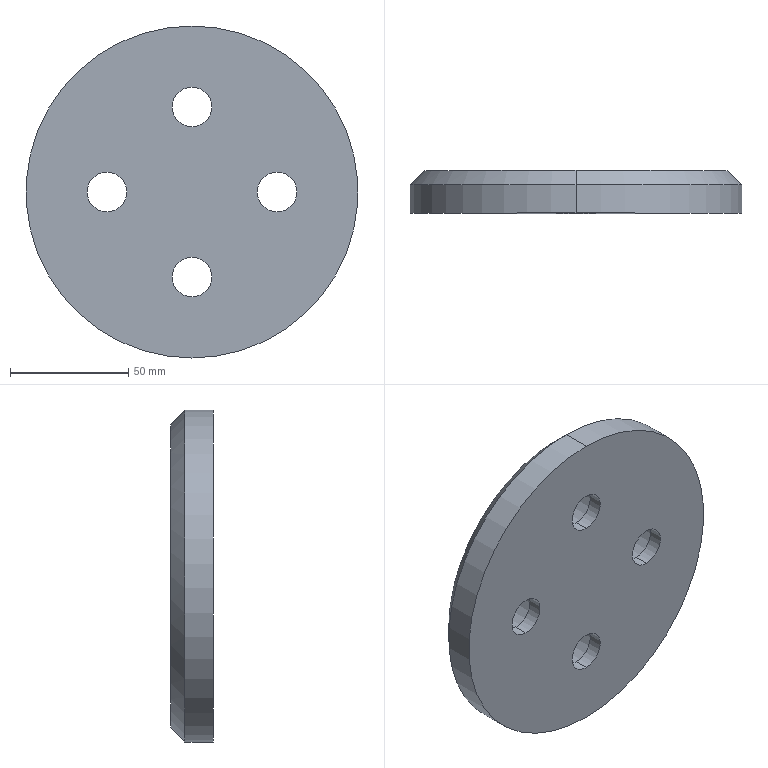Part | SolidWorks | features BaseBody 1, Scale 1 | 1 solid | 26 faces | box 140.4 x 18 x 140.4 mm | volume 234372 mm3 | cylinder 18 | plane 6 | cone 2 | commonest cylinder face diameters 16.8 x8 28.8 x8 140.4 x2
STEP:
#1=CARTESIAN_POINT('',(-36.,4.582,8.4));
#2=VERTEX_POINT('',#1);
#3=CARTESIAN_POINT('',(-36.,4.582,-8.4));
#4=VERTEX_POINT('',#3);
#5=CARTESIAN_POINT('',(-36.,4.582,0.));
#6=DIRECTION('',(0.,-1.,0.));
#7=DIRECTION('',(0.,0.,-1.));
#8=AXIS2_PLACEMENT_3D('',#5,#6,#7);
#9=CIRCLE('',#8,8.4);
#10=EDGE_CURVE('',#2,#4,#9,.T.);
#11=ORIENTED_EDGE('',*,*,#10,.F.);
#12=CARTESIAN_POINT('',(-36.,-1.418,8.4));
#13=VERTEX_POINT('',#12);
#14=CARTESIAN_POINT('',(-36.,16.582,8.4));
#15=DIRECTION('',(0.,-1.,0.));
#16=VECTOR('',#15,1000.);
#17=LINE('',#14,#16);
#18=EDGE_CURVE('',#2,#13,#17,.T.);
#19=ORIENTED_EDGE('',*,*,#18,.T.);
#20=CARTESIAN_POINT('',(-36.,-1.418,-8.4));
#21=VERTEX_POINT('',#20);
#22=CARTESIAN_POINT('',(-36.,-1.418,0.));
#23=DIRECTION('',(0.,-1.,0.));
#24=DIRECTION('',(0.,0.,-1.));
#25=AXIS2_PLACEMENT_3D('',#22,#23,#24);
#26=CIRCLE('',#25,8.4);
#27=EDGE_CURVE('',#13,#21,#26,.T.);
#28=ORIENTED_EDGE('',*,*,#27,.T.);
#29=CARTESIAN_POINT('',(-36.,16.582,-8.4));
#30=DIRECTION('',(0.,-1.,0.));
#31=VECTOR('',#30,1000.);
#32=LINE('',#29,#31);
#33=EDGE_CURVE('',#4,#21,#32,.T.);
#34=ORIENTED_EDGE('',*,*,#33,.F.);
#35=EDGE_LOOP('',(#11,#19,#28,#34));
#36=FACE_OUTER_BOUND('',#35,.T.);
#37=CARTESIAN_POINT('',(-36.,16.582,0.));
#38=DIRECTION('',(0.,-1.,0.));
#39=DIRECTION('',(0.,0.,-1.));
#40=AXIS2_PLACEMENT_3D('',#37,#38,#39);
#41=CYLINDRICAL_SURFACE('',#40,8.4);
#42=ADVANCED_FACE('',(#36),#41,.F.);
#43=CARTESIAN_POINT('',(0.,4.582,44.4));
#44=VERTEX_POINT('',#43);
#45=CARTESIAN_POINT('',(0.,4.582,27.6));
#46=VERTEX_POINT('',#45);
#47=CARTESIAN_POINT('',(0.,4.582,36.));
#48=DIRECTION('',(0.,-1.,0.));
#49=DIRECTION('',(0.,0.,-1.));
#50=AXIS2_PLACEMENT_3D('',#47,#48,#49);
#51=CIRCLE('',#50,8.4);
#52=EDGE_CURVE('',#44,#46,#51,.T.);
#53=ORIENTED_EDGE('',*,*,#52,.F.);
#54=CARTESIAN_POINT('',(0.,-1.418,44.4));
#55=VERTEX_POINT('',#54);
#56=CARTESIAN_POINT('',(0.,16.582,44.4));
#57=DIRECTION('',(0.,-1.,0.));
#58=VECTOR('',#57,1000.);
#59=LINE('',#56,#58);
#60=EDGE_CURVE('',#44,#55,#59,.T.);
#61=ORIENTED_EDGE('',*,*,#60,.T.);
#62=CARTESIAN_POINT('',(0.,-1.418,27.6));
#63=VERTEX_POINT('',#62);
#64=CARTESIAN_POINT('',(0.,-1.418,36.));
#65=DIRECTION('',(0.,-1.,0.));
#66=DIRECTION('',(0.,0.,-1.));
#67=AXIS2_PLACEMENT_3D('',#64,#65,#66);
#68=CIRCLE('',#67,8.4);
#69=EDGE_CURVE('',#55,#63,#68,.T.);
#70=ORIENTED_EDGE('',*,*,#69,.T.);
#71=CARTESIAN_POINT('',(0.,16.582,27.6));
#72=DIRECTION('',(0.,-1.,0.));
#73=VECTOR('',#72,1000.);
#74=LINE('',#71,#73);
#75=EDGE_CURVE('',#46,#63,#74,.T.);
#76=ORIENTED_EDGE('',*,*,#75,.F.);
#77=EDGE_LOOP('',(#53,#61,#70,#76));
#78=FACE_OUTER_BOUND('',#77,.T.);
#79=CARTESIAN_POINT('',(0.,16.582,36.));
#80=DIRECTION('',(0.,-1.,0.));
#81=DIRECTION('',(0.,0.,-1.));
#82=AXIS2_PLACEMENT_3D('',#79,#80,#81);
#83=CYLINDRICAL_SURFACE('',#82,8.4);
#84=ADVANCED_FACE('',(#78),#83,.F.);
#85=CARTESIAN_POINT('',(36.,4.582,8.4));
#86=VERTEX_POINT('',#85);
#87=CARTESIAN_POINT('',(36.,4.582,-8.4));
#88=VERTEX_POINT('',#87);
#89=CARTESIAN_POINT('',(36.,4.582,0.));
#90=DIRECTION('',(0.,-1.,0.));
#91=DIRECTION('',(0.,0.,-1.));
#92=AXIS2_PLACEMENT_3D('',#89,#90,#91);
#93=CIRCLE('',#92,8.4);
#94=EDGE_CURVE('',#86,#88,#93,.T.);
#95=ORIENTED_EDGE('',*,*,#94,.F.);
#96=CARTESIAN_POINT('',(36.,-1.418,8.4));
#97=VERTEX_POINT('',#96);
#98=CARTESIAN_POINT('',(36.,16.582,8.4));
#99=DIRECTION('',(0.,-1.,0.));
#100=VECTOR('',#99,1000.);
#101=LINE('',#98,#100);
#102=EDGE_CURVE('',#86,#97,#101,.T.);
#103=ORIENTED_EDGE('',*,*,#102,.T.);
#104=CARTESIAN_POINT('',(36.,-1.418,-8.4));
#105=VERTEX_POINT('',#104);
#106=CARTESIAN_POINT('',(36.,-1.418,0.));
#107=DIRECTION('',(0.,-1.,0.));
#108=DIRECTION('',(0.,0.,-1.));
#109=AXIS2_PLACEMENT_3D('',#106,#107,#108);
#110=CIRCLE('',#109,8.4);
#111=EDGE_CURVE('',#97,#105,#110,.T.);
#112=ORIENTED_EDGE('',*,*,#111,.T.);
#113=CARTESIAN_POINT('',(36.,16.582,-8.4));
#114=DIRECTION('',(0.,-1.,0.));
#115=VECTOR('',#114,1000.);
#116=LINE('',#113,#115);
#117=EDGE_CURVE('',#88,#105,#116,.T.);
#118=ORIENTED_EDGE('',*,*,#117,.F.);
#119=EDGE_LOOP('',(#95,#103,#112,#118));
#120=FACE_OUTER_BOUND('',#119,.T.);
#121=CARTESIAN_POINT('',(36.,16.582,0.));
#122=DIRECTION('',(0.,-1.,0.));
#123=DIRECTION('',(0.,0.,-1.));
#124=AXIS2_PLACEMENT_3D('',#121,#122,#123);
#125=CYLINDRICAL_SURFACE('',#124,8.4);
#126=ADVANCED_FACE('',(#120),#125,.F.);
#127=CARTESIAN_POINT('',(0.,4.582,-27.6));
#128=VERTEX_POINT('',#127);
#129=CARTESIAN_POINT('',(0.,4.582,-44.4));
#130=VERTEX_POINT('',#129);
#131=CARTESIAN_POINT('',(0.,4.582,-36.));
#132=DIRECTION('',(0.,-1.,0.));
#133=DIRECTION('',(0.,0.,-1.));
#134=AXIS2_PLACEMENT_3D('',#131,#132,#133);
#135=CIRCLE('',#134,8.4);
#136=EDGE_CURVE('',#128,#130,#135,.T.);
#137=ORIENTED_EDGE('',*,*,#136,.F.);
#138=CARTESIAN_POINT('',(0.,-1.418,-27.6));
#139=VERTEX_POINT('',#138);
#140=CARTESIAN_POINT('',(0.,16.582,-27.6));
#141=DIRECTION('',(0.,-1.,0.));
#142=VECTOR('',#141,1000.);
#143=LINE('',#140,#142);
#144=EDGE_CURVE('',#128,#139,#143,.T.);
#145=ORIENTED_EDGE('',*,*,#144,.T.);
#146=CARTESIAN_POINT('',(0.,-1.418,-44.4));
#147=VERTEX_POINT('',#146);
#148=CARTESIAN_POINT('',(0.,-1.418,-36.));
#149=DIRECTION('',(0.,-1.,0.));
#150=DIRECTION('',(0.,0.,-1.));
#151=AXIS2_PLACEMENT_3D('',#148,#149,#150);
#152=CIRCLE('',#151,8.4);
#153=EDGE_CURVE('',#139,#147,#152,.T.);
#154=ORIENTED_EDGE('',*,*,#153,.T.);
#155=CARTESIAN_POINT('',(0.,16.582,-44.4));
#156=DIRECTION('',(0.,-1.,0.));
#157=VECTOR('',#156,1000.);
#158=LINE('',#155,#157);
#159=EDGE_CURVE('',#130,#147,#158,.T.);
#160=ORIENTED_EDGE('',*,*,#159,.F.);
#161=EDGE_LOOP('',(#137,#145,#154,#160));
#162=FACE_OUTER_BOUND('',#161,.T.);
#163=CARTESIAN_POINT('',(0.,16.582,-36.));
#164=DIRECTION('',(0.,-1.,0.));
#165=DIRECTION('',(0.,0.,-1.));
#166=AXIS2_PLACEMENT_3D('',#163,#164,#165);
#167=CYLINDRICAL_SURFACE('',#166,8.4);
#168=ADVANCED_FACE('',(#162),#167,.F.);
#169=CARTESIAN_POINT('',(0.,10.582,-70.2));
#170=VERTEX_POINT('',#169);
#171=CARTESIAN_POINT('',(0.,10.582,70.2));
#172=VERTEX_POINT('',#171);
#173=CARTESIAN_POINT('',(0.,10.582,0.));
#174=DIRECTION('',(0.,-1.,0.));
#175=DIRECTION('',(0.,0.,-1.));
#176=AXIS2_PLACEMENT_3D('',#173,#174,#175);
#177=CIRCLE('',#176,70.2);
#178=EDGE_CURVE('',#170,#172,#177,.T.);
#179=ORIENTED_EDGE('',*,*,#178,.T.);
#180=CARTESIAN_POINT('',(0.,-1.418,70.2));
#181=VERTEX_POINT('',#180);
#182=CARTESIAN_POINT('',(0.,16.582,70.2));
#183=DIRECTION('',(0.,-1.,0.));
#184=VECTOR('',#183,1000.);
#185=LINE('',#182,#184);
#186=EDGE_CURVE('',#172,#181,#185,.T.);
#187=ORIENTED_EDGE('',*,*,#186,.T.);
#188=CARTESIAN_POINT('',(0.,-1.418,-70.2));
#189=VERTEX_POINT('',#188);
#190=CARTESIAN_POINT('',(0.,-1.418,0.));
#191=DIRECTION('',(0.,1.,0.));
#192=DIRECTION('',(0.,0.,-1.));
#193=AXIS2_PLACEMENT_3D('',#190,#191,#192);
#194=CIRCLE('',#193,70.2);
#195=EDGE_CURVE('',#181,#189,#194,.T.);
#196=ORIENTED_EDGE('',*,*,#195,.T.);
#197=CARTESIAN_POINT('',(0.,16.582,-70.2));
#198=DIRECTION('',(0.,-1.,0.));
#199=VECTOR('',#198,1000.);
#200=LINE('',#197,#199);
#201=EDGE_CURVE('',#170,#189,#200,.T.);
#202=ORIENTED_EDGE('',*,*,#201,.F.);
#203=EDGE_LOOP('',(#179,#187,#196,#202));
#204=FACE_OUTER_BOUND('',#203,.T.);
#205=CARTESIAN_POINT('',(0.,16.582,0.));
#206=DIRECTION('',(0.,-1.,0.));
#207=DIRECTION('',(0.,0.,-1.));
#208=AXIS2_PLACEMENT_3D('',#205,#206,#207);
#209=CYLINDRICAL_SURFACE('',#208,70.2);
#210=ADVANCED_FACE('',(#204),#209,.T.);
#211=CARTESIAN_POINT('',(0.,16.582,-64.2));
#212=VERTEX_POINT('',#211);
#213=CARTESIAN_POINT('',(0.,16.582,64.2));
#214=VERTEX_POINT('',#213);
#215=CARTESIAN_POINT('',(0.,16.582,0.));
#216=DIRECTION('',(0.,-1.,0.));
#217=DIRECTION('',(0.,0.,-1.));
#218=AXIS2_PLACEMENT_3D('',#215,#216,#217);
#219=CIRCLE('',#218,64.2);
#220=EDGE_CURVE('',#212,#214,#219,.T.);
#221=ORIENTED_EDGE('',*,*,#220,.T.);
#222=CARTESIAN_POINT('',(0.,10.582,70.2));
#223=DIRECTION('',(0.,-0.7071,0.7071));
#224=VECTOR('',#223,1000.);
#225=LINE('',#222,#224);
#226=EDGE_CURVE('',#214,#172,#225,.T.);
#227=ORIENTED_EDGE('',*,*,#226,.T.);
#228=ORIENTED_EDGE('',*,*,#178,.F.);
#229=CARTESIAN_POINT('',(0.,10.582,-70.2));
#230=DIRECTION('',(0.,-0.7071,-0.7071));
#231=VECTOR('',#230,1000.);
#232=LINE('',#229,#231);
#233=EDGE_CURVE('',#212,#170,#232,.T.);
#234=ORIENTED_EDGE('',*,*,#233,.F.);
#235=EDGE_LOOP('',(#221,#227,#228,#234));
#236=FACE_OUTER_BOUND('',#235,.T.);
#237=CARTESIAN_POINT('',(0.,10.582,0.));
#238=DIRECTION('',(0.,-1.,0.));
#239=DIRECTION('',(0.,0.,-1.));
#240=AXIS2_PLACEMENT_3D('',#237,#238,#239);
#241=CONICAL_SURFACE('',#240,70.2,0.7854);
#242=ADVANCED_FACE('',(#236),#241,.T.);
#243=CARTESIAN_POINT('',(-36.,4.582,-14.4));
#244=VERTEX_POINT('',#243);
#245=CARTESIAN_POINT('',(-36.,4.582,14.4));
#246=VERTEX_POINT('',#245);
#247=CARTESIAN_POINT('',(-36.,4.582,0.));
#248=DIRECTION('',(0.,1.,0.));
#249=DIRECTION('',(0.,0.,1.));
#250=AXIS2_PLACEMENT_3D('',#247,#248,#249);
#251=CIRCLE('',#250,14.4);
#252=EDGE_CURVE('',#244,#246,#251,.T.);
#253=ORIENTED_EDGE('',*,*,#252,.F.);
#254=CARTESIAN_POINT('',(-36.,16.582,-14.4));
#255=VERTEX_POINT('',#254);
#256=CARTESIAN_POINT('',(-36.,4.582,-14.4));
#257=DIRECTION('',(0.,1.,0.));
#258=VECTOR('',#257,1000.);
#259=LINE('',#256,#258);
#260=EDGE_CURVE('',#244,#255,#259,.T.);
#261=ORIENTED_EDGE('',*,*,#260,.T.);
#262=CARTESIAN_POINT('',(-36.,16.582,14.4));
#263=VERTEX_POINT('',#262);
#264=CARTESIAN_POINT('',(-36.,16.582,0.));
#265=DIRECTION('',(0.,-1.,0.));
#266=DIRECTION('',(0.,0.,1.));
#267=AXIS2_PLACEMENT_3D('',#264,#265,#266);
#268=CIRCLE('',#267,14.4);
#269=EDGE_CURVE('',#263,#255,#268,.T.);
#270=ORIENTED_EDGE('',*,*,#269,.F.);
#271=CARTESIAN_POINT('',(-36.,4.582,14.4));
#272=DIRECTION('',(0.,1.,0.));
#273=VECTOR('',#272,1000.);
#274=LINE('',#271,#273);
#275=EDGE_CURVE('',#246,#263,#274,.T.);
#276=ORIENTED_EDGE('',*,*,#275,.F.);
#277=EDGE_LOOP('',(#253,#261,#270,#276));
#278=FACE_OUTER_BOUND('',#277,.T.);
#279=CARTESIAN_POINT('',(-36.,4.582,0.));
#280=DIRECTION('',(0.,1.,0.));
#281=DIRECTION('',(0.,0.,1.));
#282=AXIS2_PLACEMENT_3D('',#279,#280,#281);
#283=CYLINDRICAL_SURFACE('',#282,14.4);
#284=ADVANCED_FACE('',(#278),#283,.F.);
#285=CARTESIAN_POINT('',(0.,4.582,21.6));
#286=VERTEX_POINT('',#285);
#287=CARTESIAN_POINT('',(0.,4.582,50.4));
#288=VERTEX_POINT('',#287);
#289=CARTESIAN_POINT('',(0.,4.582,36.));
#290=DIRECTION('',(0.,1.,0.));
#291=DIRECTION('',(0.,0.,1.));
#292=AXIS2_PLACEMENT_3D('',#289,#290,#291);
#293=CIRCLE('',#292,14.4);
#294=EDGE_CURVE('',#286,#288,#293,.T.);
#295=ORIENTED_EDGE('',*,*,#294,.F.);
#296=CARTESIAN_POINT('',(0.,16.582,21.6));
#297=VERTEX_POINT('',#296);
#298=CARTESIAN_POINT('',(0.,4.582,21.6));
#299=DIRECTION('',(0.,1.,0.));
#300=VECTOR('',#299,1000.);
#301=LINE('',#298,#300);
#302=EDGE_CURVE('',#286,#297,#301,.T.);
#303=ORIENTED_EDGE('',*,*,#302,.T.);
#304=CARTESIAN_POINT('',(0.,16.582,50.4));
#305=VERTEX_POINT('',#304);
#306=CARTESIAN_POINT('',(0.,16.582,36.));
#307=DIRECTION('',(0.,-1.,0.));
#308=DIRECTION('',(0.,0.,1.));
#309=AXIS2_PLACEMENT_3D('',#306,#307,#308);
#310=CIRCLE('',#309,14.4);
#311=EDGE_CURVE('',#305,#297,#310,.T.);
#312=ORIENTED_EDGE('',*,*,#311,.F.);
#313=CARTESIAN_POINT('',(0.,4.582,50.4));
#314=DIRECTION('',(0.,1.,0.));
#315=VECTOR('',#314,1000.);
#316=LINE('',#313,#315);
#317=EDGE_CURVE('',#288,#305,#316,.T.);
#318=ORIENTED_EDGE('',*,*,#317,.F.);
#319=EDGE_LOOP('',(#295,#303,#312,#318));
#320=FACE_OUTER_BOUND('',#319,.T.);
#321=CARTESIAN_POINT('',(0.,4.582,36.));
#322=DIRECTION('',(0.,1.,0.));
#323=DIRECTION('',(0.,0.,1.));
#324=AXIS2_PLACEMENT_3D('',#321,#322,#323);
#325=CYLINDRICAL_SURFACE('',#324,14.4);
#326=ADVANCED_FACE('',(#320),#325,.F.);
#327=CARTESIAN_POINT('',(36.,4.582,-14.4));
#328=VERTEX_POINT('',#327);
#329=CARTESIAN_POINT('',(36.,4.582,14.4));
#330=VERTEX_POINT('',#329);
#331=CARTESIAN_POINT('',(36.,4.582,0.));
#332=DIRECTION('',(0.,1.,0.));
#333=DIRECTION('',(0.,0.,1.));
#334=AXIS2_PLACEMENT_3D('',#331,#332,#333);
#335=CIRCLE('',#334,14.4);
#336=EDGE_CURVE('',#328,#330,#335,.T.);
#337=ORIENTED_EDGE('',*,*,#336,.F.);
#338=CARTESIAN_POINT('',(36.,16.582,-14.4));
#339=VERTEX_POINT('',#338);
#340=CARTESIAN_POINT('',(36.,4.582,-14.4));
#341=DIRECTION('',(0.,1.,0.));
#342=VECTOR('',#341,1000.);
#343=LINE('',#340,#342);
#344=EDGE_CURVE('',#328,#339,#343,.T.);
#345=ORIENTED_EDGE('',*,*,#344,.T.);
#346=CARTESIAN_POINT('',(36.,16.582,14.4));
#347=VERTEX_POINT('',#346);
#348=CARTESIAN_POINT('',(36.,16.582,0.));
#349=DIRECTION('',(0.,-1.,0.));
#350=DIRECTION('',(0.,0.,1.));
#351=AXIS2_PLACEMENT_3D('',#348,#349,#350);
#352=CIRCLE('',#351,14.4);
#353=EDGE_CURVE('',#347,#339,#352,.T.);
#354=ORIENTED_EDGE('',*,*,#353,.F.);
#355=CARTESIAN_POINT('',(36.,4.582,14.4));
#356=DIRECTION('',(0.,1.,0.));
#357=VECTOR('',#356,1000.);
#358=LINE('',#355,#357);
#359=EDGE_CURVE('',#330,#347,#358,.T.);
#360=ORIENTED_EDGE('',*,*,#359,.F.);
#361=EDGE_LOOP('',(#337,#345,#354,#360));
#362=FACE_OUTER_BOUND('',#361,.T.);
#363=CARTESIAN_POINT('',(36.,4.582,0.));
#364=DIRECTION('',(0.,1.,0.));
#365=DIRECTION('',(0.,0.,1.));
#366=AXIS2_PLACEMENT_3D('',#363,#364,#365);
#367=CYLINDRICAL_SURFACE('',#366,14.4);
#368=ADVANCED_FACE('',(#362),#367,.F.);
#369=CARTESIAN_POINT('',(0.,4.582,-50.4));
#370=VERTEX_POINT('',#369);
#371=CARTESIAN_POINT('',(0.,4.582,-21.6));
#372=VERTEX_POINT('',#371);
#373=CARTESIAN_POINT('',(0.,4.582,-36.));
#374=DIRECTION('',(0.,1.,0.));
#375=DIRECTION('',(0.,0.,1.));
#376=AXIS2_PLACEMENT_3D('',#373,#374,#375);
#377=CIRCLE('',#376,14.4);
#378=EDGE_CURVE('',#370,#372,#377,.T.);
#379=ORIENTED_EDGE('',*,*,#378,.F.);
#380=CARTESIAN_POINT('',(0.,16.582,-50.4));
#381=VERTEX_POINT('',#380);
#382=CARTESIAN_POINT('',(0.,4.582,-50.4));
#383=DIRECTION('',(0.,1.,0.));
#384=VECTOR('',#383,1000.);
#385=LINE('',#382,#384);
#386=EDGE_CURVE('',#370,#381,#385,.T.);
#387=ORIENTED_EDGE('',*,*,#386,.T.);
#388=CARTESIAN_POINT('',(0.,16.582,-21.6));
#389=VERTEX_POINT('',#388);
#390=CARTESIAN_POINT('',(0.,16.582,-36.));
#391=DIRECTION('',(0.,-1.,0.));
#392=DIRECTION('',(0.,0.,1.));
#393=AXIS2_PLACEMENT_3D('',#390,#391,#392);
#394=CIRCLE('',#393,14.4);
#395=EDGE_CURVE('',#389,#381,#394,.T.);
#396=ORIENTED_EDGE('',*,*,#395,.F.);
#397=CARTESIAN_POINT('',(0.,4.582,-21.6));
#398=DIRECTION('',(0.,1.,0.));
#399=VECTOR('',#398,1000.);
#400=LINE('',#397,#399);
#401=EDGE_CURVE('',#372,#389,#400,.T.);
#402=ORIENTED_EDGE('',*,*,#401,.F.);
#403=EDGE_LOOP('',(#379,#387,#396,#402));
#404=FACE_OUTER_BOUND('',#403,.T.);
#405=CARTESIAN_POINT('',(0.,4.582,-36.));
#406=DIRECTION('',(0.,1.,0.));
#407=DIRECTION('',(0.,0.,1.));
#408=AXIS2_PLACEMENT_3D('',#405,#406,#407);
#409=CYLINDRICAL_SURFACE('',#408,14.4);
#410=ADVANCED_FACE('',(#404),#409,.F.);
#411=CARTESIAN_POINT('',(-36.,-1.418,0.));
#412=DIRECTION('',(0.,-1.,0.));
#413=DIRECTION('',(0.,0.,-1.));
#414=AXIS2_PLACEMENT_3D('',#411,#412,#413);
#415=CIRCLE('',#414,8.4);
#416=EDGE_CURVE('',#21,#13,#415,.T.);
#417=ORIENTED_EDGE('',*,*,#416,.F.);
#418=ORIENTED_EDGE('',*,*,#27,.F.);
#419=EDGE_LOOP('',(#417,#418));
#420=FACE_BOUND('',#419,.T.);
#421=CARTESIAN_POINT('',(0.,-1.418,36.));
#422=DIRECTION('',(0.,-1.,0.));
#423=DIRECTION('',(0.,0.,-1.));
#424=AXIS2_PLACEMENT_3D('',#421,#422,#423);
#425=CIRCLE('',#424,8.4);
#426=EDGE_CURVE('',#63,#55,#425,.T.);
#427=ORIENTED_EDGE('',*,*,#426,.F.);
#428=ORIENTED_EDGE('',*,*,#69,.F.);
#429=EDGE_LOOP('',(#427,#428));
#430=FACE_BOUND('',#429,.T.);
#431=CARTESIAN_POINT('',(36.,-1.418,0.));
#432=DIRECTION('',(0.,-1.,0.));
#433=DIRECTION('',(0.,0.,-1.));
#434=AXIS2_PLACEMENT_3D('',#431,#432,#433);
#435=CIRCLE('',#434,8.4);
#436=EDGE_CURVE('',#105,#97,#435,.T.);
#437=ORIENTED_EDGE('',*,*,#436,.F.);
#438=ORIENTED_EDGE('',*,*,#111,.F.);
#439=EDGE_LOOP('',(#437,#438));
#440=FACE_BOUND('',#439,.T.);
#441=CARTESIAN_POINT('',(0.,-1.418,-36.));
#442=DIRECTION('',(0.,-1.,0.));
#443=DIRECTION('',(0.,0.,-1.));
#444=AXIS2_PLACEMENT_3D('',#441,#442,#443);
#445=CIRCLE('',#444,8.4);
#446=EDGE_CURVE('',#147,#139,#445,.T.);
#447=ORIENTED_EDGE('',*,*,#446,.F.);
#448=ORIENTED_EDGE('',*,*,#153,.F.);
#449=EDGE_LOOP('',(#447,#448));
#450=FACE_BOUND('',#449,.T.);
#451=CARTESIAN_POINT('',(0.,-1.418,0.));
#452=DIRECTION('',(0.,1.,0.));
#453=DIRECTION('',(0.,0.,-1.));
#454=AXIS2_PLACEMENT_3D('',#451,#452,#453);
#455=CIRCLE('',#454,70.2);
#456=EDGE_CURVE('',#189,#181,#455,.T.);
#457=ORIENTED_EDGE('',*,*,#456,.F.);
#458=ORIENTED_EDGE('',*,*,#195,.F.);
#459=EDGE_LOOP('',(#457,#458));
#460=FACE_OUTER_BOUND('',#459,.T.);
#461=CARTESIAN_POINT('',(0.,-1.418,0.));
#462=DIRECTION('',(0.,1.,0.));
#463=DIRECTION('',(0.,0.,1.));
#464=AXIS2_PLACEMENT_3D('',#461,#462,#463);
#465=PLANE('',#464);
#466=ADVANCED_FACE('',(#420,#430,#440,#450,#460),#465,.F.);
#467=ORIENTED_EDGE('',*,*,#18,.F.);
#468=CARTESIAN_POINT('',(-36.,4.582,0.));
#469=DIRECTION('',(0.,-1.,0.));
#470=DIRECTION('',(0.,0.,-1.));
#471=AXIS2_PLACEMENT_3D('',#468,#469,#470);
#472=CIRCLE('',#471,8.4);
#473=EDGE_CURVE('',#4,#2,#472,.T.);
#474=ORIENTED_EDGE('',*,*,#473,.F.);
#475=ORIENTED_EDGE('',*,*,#33,.T.);
#476=ORIENTED_EDGE('',*,*,#416,.T.);
#477=EDGE_LOOP('',(#467,#474,#475,#476));
#478=FACE_OUTER_BOUND('',#477,.T.);
#479=CARTESIAN_POINT('',(-36.,16.582,0.));
#480=DIRECTION('',(0.,-1.,0.));
#481=DIRECTION('',(0.,0.,-1.));
#482=AXIS2_PLACEMENT_3D('',#479,#480,#481);
#483=CYLINDRICAL_SURFACE('',#482,8.4);
#484=ADVANCED_FACE('',(#478),#483,.F.);
#485=ORIENTED_EDGE('',*,*,#60,.F.);
#486=CARTESIAN_POINT('',(0.,4.582,36.));
#487=DIRECTION('',(0.,-1.,0.));
#488=DIRECTION('',(0.,0.,-1.));
#489=AXIS2_PLACEMENT_3D('',#486,#487,#488);
#490=CIRCLE('',#489,8.4);
#491=EDGE_CURVE('',#46,#44,#490,.T.);
#492=ORIENTED_EDGE('',*,*,#491,.F.);
#493=ORIENTED_EDGE('',*,*,#75,.T.);
#494=ORIENTED_EDGE('',*,*,#426,.T.);
#495=EDGE_LOOP('',(#485,#492,#493,#494));
#496=FACE_OUTER_BOUND('',#495,.T.);
#497=CARTESIAN_POINT('',(0.,16.582,36.));
#498=DIRECTION('',(0.,-1.,0.));
#499=DIRECTION('',(0.,0.,-1.));
#500=AXIS2_PLACEMENT_3D('',#497,#498,#499);
#501=CYLINDRICAL_SURFACE('',#500,8.4);
#502=ADVANCED_FACE('',(#496),#501,.F.);
#503=ORIENTED_EDGE('',*,*,#102,.F.);
#504=CARTESIAN_POINT('',(36.,4.582,0.));
#505=DIRECTION('',(0.,-1.,0.));
#506=DIRECTION('',(0.,0.,-1.));
#507=AXIS2_PLACEMENT_3D('',#504,#505,#506);
#508=CIRCLE('',#507,8.4);
#509=EDGE_CURVE('',#88,#86,#508,.T.);
#510=ORIENTED_EDGE('',*,*,#509,.F.);
#511=ORIENTED_EDGE('',*,*,#117,.T.);
#512=ORIENTED_EDGE('',*,*,#436,.T.);
#513=EDGE_LOOP('',(#503,#510,#511,#512));
#514=FACE_OUTER_BOUND('',#513,.T.);
#515=CARTESIAN_POINT('',(36.,16.582,0.));
#516=DIRECTION('',(0.,-1.,0.));
#517=DIRECTION('',(0.,0.,-1.));
#518=AXIS2_PLACEMENT_3D('',#515,#516,#517);
#519=CYLINDRICAL_SURFACE('',#518,8.4);
#520=ADVANCED_FACE('',(#514),#519,.F.);
#521=ORIENTED_EDGE('',*,*,#144,.F.);
#522=CARTESIAN_POINT('',(0.,4.582,-36.));
#523=DIRECTION('',(0.,-1.,0.));
#524=DIRECTION('',(0.,0.,-1.));
#525=AXIS2_PLACEMENT_3D('',#522,#523,#524);
#526=CIRCLE('',#525,8.4);
#527=EDGE_CURVE('',#130,#128,#526,.T.);
#528=ORIENTED_EDGE('',*,*,#527,.F.);
#529=ORIENTED_EDGE('',*,*,#159,.T.);
#530=ORIENTED_EDGE('',*,*,#446,.T.);
#531=EDGE_LOOP('',(#521,#528,#529,#530));
#532=FACE_OUTER_BOUND('',#531,.T.);
#533=CARTESIAN_POINT('',(0.,16.582,-36.));
#534=DIRECTION('',(0.,-1.,0.));
#535=DIRECTION('',(0.,0.,-1.));
#536=AXIS2_PLACEMENT_3D('',#533,#534,#535);
#537=CYLINDRICAL_SURFACE('',#536,8.4);
#538=ADVANCED_FACE('',(#532),#537,.F.);
#539=ORIENTED_EDGE('',*,*,#186,.F.);
#540=CARTESIAN_POINT('',(0.,10.582,0.));
#541=DIRECTION('',(0.,-1.,0.));
#542=DIRECTION('',(0.,0.,-1.));
#543=AXIS2_PLACEMENT_3D('',#540,#541,#542);
#544=CIRCLE('',#543,70.2);
#545=EDGE_CURVE('',#172,#170,#544,.T.);
#546=ORIENTED_EDGE('',*,*,#545,.T.);
#547=ORIENTED_EDGE('',*,*,#201,.T.);
#548=ORIENTED_EDGE('',*,*,#456,.T.);
#549=EDGE_LOOP('',(#539,#546,#547,#548));
#550=FACE_OUTER_BOUND('',#549,.T.);
#551=CARTESIAN_POINT('',(0.,16.582,0.));
#552=DIRECTION('',(0.,-1.,0.));
#553=DIRECTION('',(0.,0.,-1.));
#554=AXIS2_PLACEMENT_3D('',#551,#552,#553);
#555=CYLINDRICAL_SURFACE('',#554,70.2);
#556=ADVANCED_FACE('',(#550),#555,.T.);
#557=CARTESIAN_POINT('',(-36.,4.582,0.));
#558=DIRECTION('',(0.,1.,0.));
#559=DIRECTION('',(0.,0.,1.));
#560=AXIS2_PLACEMENT_3D('',#557,#558,#559);
#561=CIRCLE('',#560,14.4);
#562=EDGE_CURVE('',#246,#244,#561,.T.);
#563=ORIENTED_EDGE('',*,*,#562,.T.);
#564=ORIENTED_EDGE('',*,*,#252,.T.);
#565=EDGE_LOOP('',(#563,#564));
#566=FACE_OUTER_BOUND('',#565,.T.);
#567=ORIENTED_EDGE('',*,*,#473,.T.);
#568=ORIENTED_EDGE('',*,*,#10,.T.);
#569=EDGE_LOOP('',(#567,#568));
#570=FACE_BOUND('',#569,.T.);
#571=CARTESIAN_POINT('',(-36.,4.582,0.));
#572=DIRECTION('',(0.,1.,0.));
#573=DIRECTION('',(0.,0.,1.));
#574=AXIS2_PLACEMENT_3D('',#571,#572,#573);
#575=PLANE('',#574);
#576=ADVANCED_FACE('',(#566,#570),#575,.T.);
#577=CARTESIAN_POINT('',(0.,4.582,36.));
#578=DIRECTION('',(0.,1.,0.));
#579=DIRECTION('',(0.,0.,1.));
#580=AXIS2_PLACEMENT_3D('',#577,#578,#579);
#581=CIRCLE('',#580,14.4);
#582=EDGE_CURVE('',#288,#286,#581,.T.);
#583=ORIENTED_EDGE('',*,*,#582,.T.);
#584=ORIENTED_EDGE('',*,*,#294,.T.);
#585=EDGE_LOOP('',(#583,#584));
#586=FACE_OUTER_BOUND('',#585,.T.);
#587=ORIENTED_EDGE('',*,*,#491,.T.);
#588=ORIENTED_EDGE('',*,*,#52,.T.);
#589=EDGE_LOOP('',(#587,#588));
#590=FACE_BOUND('',#589,.T.);
#591=CARTESIAN_POINT('',(0.,4.582,36.));
#592=DIRECTION('',(0.,1.,0.));
#593=DIRECTION('',(0.,0.,1.));
#594=AXIS2_PLACEMENT_3D('',#591,#592,#593);
#595=PLANE('',#594);
#596=ADVANCED_FACE('',(#586,#590),#595,.T.);
#597=CARTESIAN_POINT('',(36.,4.582,0.));
#598=DIRECTION('',(0.,1.,0.));
#599=DIRECTION('',(0.,0.,1.));
#600=AXIS2_PLACEMENT_3D('',#597,#598,#599);
#601=CIRCLE('',#600,14.4);
#602=EDGE_CURVE('',#330,#328,#601,.T.);
#603=ORIENTED_EDGE('',*,*,#602,.T.);
#604=ORIENTED_EDGE('',*,*,#336,.T.);
#605=EDGE_LOOP('',(#603,#604));
#606=FACE_OUTER_BOUND('',#605,.T.);
#607=ORIENTED_EDGE('',*,*,#509,.T.);
#608=ORIENTED_EDGE('',*,*,#94,.T.);
#609=EDGE_LOOP('',(#607,#608));
#610=FACE_BOUND('',#609,.T.);
#611=CARTESIAN_POINT('',(36.,4.582,0.));
#612=DIRECTION('',(0.,1.,0.));
#613=DIRECTION('',(0.,0.,1.));
#614=AXIS2_PLACEMENT_3D('',#611,#612,#613);
#615=PLANE('',#614);
#616=ADVANCED_FACE('',(#606,#610),#615,.T.);
#617=CARTESIAN_POINT('',(0.,4.582,-36.));
#618=DIRECTION('',(0.,1.,0.));
#619=DIRECTION('',(0.,0.,1.));
#620=AXIS2_PLACEMENT_3D('',#617,#618,#619);
#621=CIRCLE('',#620,14.4);
#622=EDGE_CURVE('',#372,#370,#621,.T.);
#623=ORIENTED_EDGE('',*,*,#622,.T.);
#624=ORIENTED_EDGE('',*,*,#378,.T.);
#625=EDGE_LOOP('',(#623,#624));
#626=FACE_OUTER_BOUND('',#625,.T.);
#627=ORIENTED_EDGE('',*,*,#527,.T.);
#628=ORIENTED_EDGE('',*,*,#136,.T.);
#629=EDGE_LOOP('',(#627,#628));
#630=FACE_BOUND('',#629,.T.);
#631=CARTESIAN_POINT('',(0.,4.582,-36.));
#632=DIRECTION('',(0.,1.,0.));
#633=DIRECTION('',(0.,0.,1.));
#634=AXIS2_PLACEMENT_3D('',#631,#632,#633);
#635=PLANE('',#634);
#636=ADVANCED_FACE('',(#626,#630),#635,.T.);
#637=ORIENTED_EDGE('',*,*,#226,.F.);
#638=CARTESIAN_POINT('',(0.,16.582,0.));
#639=DIRECTION('',(0.,-1.,0.));
#640=DIRECTION('',(0.,0.,-1.));
#641=AXIS2_PLACEMENT_3D('',#638,#639,#640);
#642=CIRCLE('',#641,64.2);
#643=EDGE_CURVE('',#214,#212,#642,.T.);
#644=ORIENTED_EDGE('',*,*,#643,.T.);
#645=ORIENTED_EDGE('',*,*,#233,.T.);
#646=ORIENTED_EDGE('',*,*,#545,.F.);
#647=EDGE_LOOP('',(#637,#644,#645,#646));
#648=FACE_OUTER_BOUND('',#647,.T.);
#649=CARTESIAN_POINT('',(0.,10.582,0.));
#650=DIRECTION('',(0.,-1.,0.));
#651=DIRECTION('',(0.,0.,-1.));
#652=AXIS2_PLACEMENT_3D('',#649,#650,#651);
#653=CONICAL_SURFACE('',#652,70.2,0.7854);
#654=ADVANCED_FACE('',(#648),#653,.T.);
#655=ORIENTED_EDGE('',*,*,#260,.F.);
#656=ORIENTED_EDGE('',*,*,#562,.F.);
#657=ORIENTED_EDGE('',*,*,#275,.T.);
#658=CARTESIAN_POINT('',(-36.,16.582,0.));
#659=DIRECTION('',(0.,-1.,0.));
#660=DIRECTION('',(0.,0.,1.));
#661=AXIS2_PLACEMENT_3D('',#658,#659,#660);
#662=CIRCLE('',#661,14.4);
#663=EDGE_CURVE('',#255,#263,#662,.T.);
#664=ORIENTED_EDGE('',*,*,#663,.F.);
#665=EDGE_LOOP('',(#655,#656,#657,#664));
#666=FACE_OUTER_BOUND('',#665,.T.);
#667=CARTESIAN_POINT('',(-36.,4.582,0.));
#668=DIRECTION('',(0.,1.,0.));
#669=DIRECTION('',(0.,0.,1.));
#670=AXIS2_PLACEMENT_3D('',#667,#668,#669);
#671=CYLINDRICAL_SURFACE('',#670,14.4);
#672=ADVANCED_FACE('',(#666),#671,.F.);
#673=ORIENTED_EDGE('',*,*,#302,.F.);
#674=ORIENTED_EDGE('',*,*,#582,.F.);
#675=ORIENTED_EDGE('',*,*,#317,.T.);
#676=CARTESIAN_POINT('',(0.,16.582,36.));
#677=DIRECTION('',(0.,-1.,0.));
#678=DIRECTION('',(0.,0.,1.));
#679=AXIS2_PLACEMENT_3D('',#676,#677,#678);
#680=CIRCLE('',#679,14.4);
#681=EDGE_CURVE('',#297,#305,#680,.T.);
#682=ORIENTED_EDGE('',*,*,#681,.F.);
#683=EDGE_LOOP('',(#673,#674,#675,#682));
#684=FACE_OUTER_BOUND('',#683,.T.);
#685=CARTESIAN_POINT('',(0.,4.582,36.));
#686=DIRECTION('',(0.,1.,0.));
#687=DIRECTION('',(0.,0.,1.));
#688=AXIS2_PLACEMENT_3D('',#685,#686,#687);
#689=CYLINDRICAL_SURFACE('',#688,14.4);
#690=ADVANCED_FACE('',(#684),#689,.F.);
#691=ORIENTED_EDGE('',*,*,#344,.F.);
#692=ORIENTED_EDGE('',*,*,#602,.F.);
#693=ORIENTED_EDGE('',*,*,#359,.T.);
#694=CARTESIAN_POINT('',(36.,16.582,0.));
#695=DIRECTION('',(0.,-1.,0.));
#696=DIRECTION('',(0.,0.,1.));
#697=AXIS2_PLACEMENT_3D('',#694,#695,#696);
#698=CIRCLE('',#697,14.4);
#699=EDGE_CURVE('',#339,#347,#698,.T.);
#700=ORIENTED_EDGE('',*,*,#699,.F.);
#701=EDGE_LOOP('',(#691,#692,#693,#700));
#702=FACE_OUTER_BOUND('',#701,.T.);
#703=CARTESIAN_POINT('',(36.,4.582,0.));
#704=DIRECTION('',(0.,1.,0.));
#705=DIRECTION('',(0.,0.,1.));
#706=AXIS2_PLACEMENT_3D('',#703,#704,#705);
#707=CYLINDRICAL_SURFACE('',#706,14.4);
#708=ADVANCED_FACE('',(#702),#707,.F.);
#709=ORIENTED_EDGE('',*,*,#386,.F.);
#710=ORIENTED_EDGE('',*,*,#622,.F.);
#711=ORIENTED_EDGE('',*,*,#401,.T.);
#712=CARTESIAN_POINT('',(0.,16.582,-36.));
#713=DIRECTION('',(0.,-1.,0.));
#714=DIRECTION('',(0.,0.,1.));
#715=AXIS2_PLACEMENT_3D('',#712,#713,#714);
#716=CIRCLE('',#715,14.4);
#717=EDGE_CURVE('',#381,#389,#716,.T.);
#718=ORIENTED_EDGE('',*,*,#717,.F.);
#719=EDGE_LOOP('',(#709,#710,#711,#718));
#720=FACE_OUTER_BOUND('',#719,.T.);
#721=CARTESIAN_POINT('',(0.,4.582,-36.));
#722=DIRECTION('',(0.,1.,0.));
#723=DIRECTION('',(0.,0.,1.));
#724=AXIS2_PLACEMENT_3D('',#721,#722,#723);
#725=CYLINDRICAL_SURFACE('',#724,14.4);
#726=ADVANCED_FACE('',(#720),#725,.F.);
#727=ORIENTED_EDGE('',*,*,#269,.T.);
#728=ORIENTED_EDGE('',*,*,#663,.T.);
#729=EDGE_LOOP('',(#727,#728));
#730=FACE_BOUND('',#729,.T.);
#731=ORIENTED_EDGE('',*,*,#311,.T.);
#732=ORIENTED_EDGE('',*,*,#681,.T.);
#733=EDGE_LOOP('',(#731,#732));
#734=FACE_BOUND('',#733,.T.);
#735=ORIENTED_EDGE('',*,*,#353,.T.);
#736=ORIENTED_EDGE('',*,*,#699,.T.);
#737=EDGE_LOOP('',(#735,#736));
#738=FACE_BOUND('',#737,.T.);
#739=ORIENTED_EDGE('',*,*,#395,.T.);
#740=ORIENTED_EDGE('',*,*,#717,.T.);
#741=EDGE_LOOP('',(#739,#740));
#742=FACE_BOUND('',#741,.T.);
#743=ORIENTED_EDGE('',*,*,#220,.F.);
#744=ORIENTED_EDGE('',*,*,#643,.F.);
#745=EDGE_LOOP('',(#743,#744));
#746=FACE_OUTER_BOUND('',#745,.T.);
#747=CARTESIAN_POINT('',(0.,16.582,0.));
#748=DIRECTION('',(0.,1.,0.));
#749=DIRECTION('',(0.,0.,1.));
#750=AXIS2_PLACEMENT_3D('',#747,#748,#749);
#751=PLANE('',#750);
#752=ADVANCED_FACE('',(#730,#734,#738,#742,#746),#751,.T.);
#753=CLOSED_SHELL('',(#42,#84,#126,#168,#210,#242,#284,#326,#368,#410,#466,#484,#502,#520,#538,#556,#576,#596,#616,#636,#654,#672,#690,#708,#726,#752));
#754=MANIFOLD_SOLID_BREP('',#753);
#755=CARTESIAN_POINT('',(0.,0.,0.));
#756=DIRECTION('',(0.,0.,1.));
#757=DIRECTION('',(1.,0.,0.));
#758=AXIS2_PLACEMENT_3D('',#755,#756,#757);
#759=(LENGTH_UNIT()NAMED_UNIT(*)SI_UNIT(.MILLI.,.METRE.));
#760=UNCERTAINTY_MEASURE_WITH_UNIT(LENGTH_MEASURE(0.00001),#759,'','');
#761=(NAMED_UNIT(*)PLANE_ANGLE_UNIT()SI_UNIT($,.RADIAN.));
#762=(NAMED_UNIT(*)SI_UNIT($,.STERADIAN.)SOLID_ANGLE_UNIT());
#763=(GEOMETRIC_REPRESENTATION_CONTEXT(3)GLOBAL_UNCERTAINTY_ASSIGNED_CONTEXT((#760))GLOBAL_UNIT_ASSIGNED_CONTEXT((#759,#761,#762))REPRESENTATION_CONTEXT('',''));
#764=ADVANCED_BREP_SHAPE_REPRESENTATION('',(#754,#758),#763);